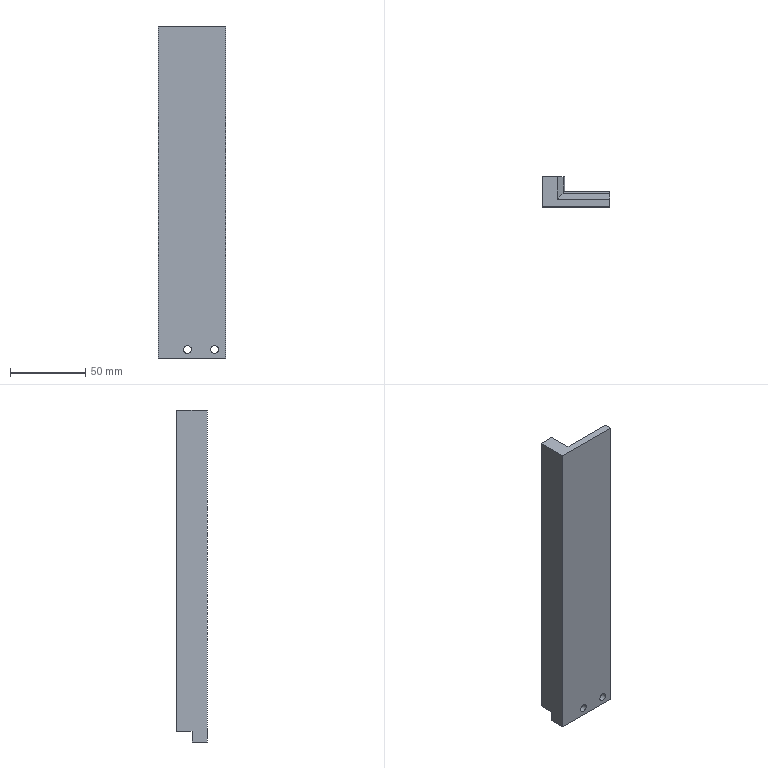Part | STEP file | Tube feed_id110_x_t | 1 solid | 19 faces | box 45 x 20 x 220 mm | volume 129034 mm3 | plane 13 | cylinder 6 | commonest cylinder face diameters 5.2 x2 8.5 x2 20 x2
STEP:
#1=CARTESIAN_POINT('',(0.,0.,0.));
#2=DIRECTION('',(0.,0.,1.));
#3=DIRECTION('',(1.,0.,0.));
#4=AXIS2_PLACEMENT_3D('',#1,#2,#3);
#5=CARTESIAN_POINT('',(-4.,404.936,201.639));
#6=VERTEX_POINT('',#5);
#7=CARTESIAN_POINT('',(-4.,404.936,1.));
#8=VERTEX_POINT('',#7);
#9=CARTESIAN_POINT('',(-4.,404.936,140.));
#10=DIRECTION('',(0.,0.,-1.));
#11=VECTOR('',#10,1.);
#12=LINE('',#9,#11);
#13=CARTESIAN_POINT('',(-4.,411.936,140.));
#14=DIRECTION('',(-1.,0.,0.));
#15=DIRECTION('',(0.,0.,1.));
#16=AXIS2_PLACEMENT_3D('',#13,#14,#15);
#17=PLANE('',#16);
#18=CARTESIAN_POINT('',(0.,-7.));
#19=DIRECTION('',(-1.,0.));
#20=VECTOR('',#19,1.);
#21=LINE('',#18,#20);
#22=(GEOMETRIC_REPRESENTATION_CONTEXT(2)PARAMETRIC_REPRESENTATION_CONTEXT()REPRESENTATION_CONTEXT('',''));
#23=DEFINITIONAL_REPRESENTATION('',(#21),#22);
#24=PCURVE('',#17,#23);
#25=CARTESIAN_POINT('',(-81.505,404.936,329.));
#26=DIRECTION('',(0.,1.,0.));
#27=DIRECTION('',(0.,0.,1.));
#28=AXIS2_PLACEMENT_3D('',#25,#26,#27);
#29=PLANE('',#28);
#30=CARTESIAN_POINT('',(-189.,77.505));
#31=DIRECTION('',(-1.,0.));
#32=VECTOR('',#31,1.);
#33=LINE('',#30,#32);
#34=(GEOMETRIC_REPRESENTATION_CONTEXT(2)PARAMETRIC_REPRESENTATION_CONTEXT()REPRESENTATION_CONTEXT('',''));
#35=DEFINITIONAL_REPRESENTATION('',(#33),#34);
#36=PCURVE('',#29,#35);
#37=SURFACE_CURVE('',#12,(#24,#36),.PCURVE_S1.);
#38=EDGE_CURVE('',#6,#8,#37,.T.);
#39=ORIENTED_EDGE('',*,*,#38,.F.);
#40=CARTESIAN_POINT('',(-4.,394.936,201.639));
#41=VERTEX_POINT('',#40);
#42=CARTESIAN_POINT('',(-4.,394.936,201.639));
#43=DIRECTION('',(0.,-1.,0.));
#44=VECTOR('',#43,1.);
#45=LINE('',#42,#44);
#46=CARTESIAN_POINT('',(61.639,-17.));
#47=DIRECTION('',(0.,-1.));
#48=VECTOR('',#47,1.);
#49=LINE('',#46,#48);
#50=(GEOMETRIC_REPRESENTATION_CONTEXT(2)PARAMETRIC_REPRESENTATION_CONTEXT()REPRESENTATION_CONTEXT('',''));
#51=DEFINITIONAL_REPRESENTATION('',(#49),#50);
#52=PCURVE('',#17,#51);
#53=CARTESIAN_POINT('',(-14.,411.936,201.639));
#54=DIRECTION('',(0.,1.,0.));
#55=DIRECTION('',(-1.,0.,0.));
#56=AXIS2_PLACEMENT_3D('',#53,#54,#55);
#57=CYLINDRICAL_SURFACE('',#56,10.);
#58=CARTESIAN_POINT('',(3.142,-17.));
#59=DIRECTION('',(0.,-1.));
#60=VECTOR('',#59,1.);
#61=LINE('',#58,#60);
#62=(GEOMETRIC_REPRESENTATION_CONTEXT(2)PARAMETRIC_REPRESENTATION_CONTEXT()REPRESENTATION_CONTEXT('',''));
#63=DEFINITIONAL_REPRESENTATION('',(#61),#62);
#64=PCURVE('',#57,#63);
#65=SURFACE_CURVE('',#45,(#52,#64),.PCURVE_S1.);
#66=EDGE_CURVE('',#6,#41,#65,.T.);
#67=ORIENTED_EDGE('',*,*,#66,.T.);
#68=CARTESIAN_POINT('',(-4.,394.936,1.));
#69=VERTEX_POINT('',#68);
#70=CARTESIAN_POINT('',(-4.,394.936,140.));
#71=DIRECTION('',(0.,0.,-1.));
#72=VECTOR('',#71,1.);
#73=LINE('',#70,#72);
#74=CARTESIAN_POINT('',(0.,-17.));
#75=DIRECTION('',(-1.,0.));
#76=VECTOR('',#75,1.);
#77=LINE('',#74,#76);
#78=(GEOMETRIC_REPRESENTATION_CONTEXT(2)PARAMETRIC_REPRESENTATION_CONTEXT()REPRESENTATION_CONTEXT('',''));
#79=DEFINITIONAL_REPRESENTATION('',(#77),#78);
#80=PCURVE('',#17,#79);
#81=CARTESIAN_POINT('',(21.,394.936,140.));
#82=DIRECTION('',(0.,-1.,0.));
#83=DIRECTION('',(0.,0.,-1.));
#84=AXIS2_PLACEMENT_3D('',#81,#82,#83);
#85=PLANE('',#84);
#86=CARTESIAN_POINT('',(0.,-25.));
#87=DIRECTION('',(1.,0.));
#88=VECTOR('',#87,1.);
#89=LINE('',#86,#88);
#90=(GEOMETRIC_REPRESENTATION_CONTEXT(2)PARAMETRIC_REPRESENTATION_CONTEXT()REPRESENTATION_CONTEXT('',''));
#91=DEFINITIONAL_REPRESENTATION('',(#89),#90);
#92=PCURVE('',#85,#91);
#93=SURFACE_CURVE('',#73,(#80,#92),.PCURVE_S1.);
#94=EDGE_CURVE('',#41,#69,#93,.T.);
#95=ORIENTED_EDGE('',*,*,#94,.T.);
#96=CARTESIAN_POINT('',(-4.,0.,1.));
#97=DIRECTION('',(0.,-1.,0.));
#98=VECTOR('',#97,1.);
#99=LINE('',#96,#98);
#100=CARTESIAN_POINT('',(-139.,-411.936));
#101=DIRECTION('',(0.,-1.));
#102=VECTOR('',#101,1.);
#103=LINE('',#100,#102);
#104=(GEOMETRIC_REPRESENTATION_CONTEXT(2)PARAMETRIC_REPRESENTATION_CONTEXT()REPRESENTATION_CONTEXT('',''));
#105=DEFINITIONAL_REPRESENTATION('',(#103),#104);
#106=PCURVE('',#17,#105);
#107=CARTESIAN_POINT('',(0.,0.,1.));
#108=DIRECTION('',(0.,0.,1.));
#109=DIRECTION('',(0.,-1.,0.));
#110=AXIS2_PLACEMENT_3D('',#107,#108,#109);
#111=PLANE('',#110);
#112=CARTESIAN_POINT('',(0.,-4.));
#113=DIRECTION('',(1.,0.));
#114=VECTOR('',#113,1.);
#115=LINE('',#112,#114);
#116=(GEOMETRIC_REPRESENTATION_CONTEXT(2)PARAMETRIC_REPRESENTATION_CONTEXT()REPRESENTATION_CONTEXT('',''));
#117=DEFINITIONAL_REPRESENTATION('',(#115),#116);
#118=PCURVE('',#111,#117);
#119=SURFACE_CURVE('',#99,(#106,#118),.PCURVE_S1.);
#120=EDGE_CURVE('',#8,#69,#119,.T.);
#121=ORIENTED_EDGE('',*,*,#120,.F.);
#122=EDGE_LOOP('',(#39,#67,#95,#121));
#123=FACE_BOUND('',#122,.T.);
#124=ADVANCED_FACE('',(#123),#17,.F.);
#125=CARTESIAN_POINT('',(-19.,394.936,-6.));
#126=VERTEX_POINT('',#125);
#127=CARTESIAN_POINT('',(-19.,384.936,-6.));
#128=VERTEX_POINT('',#127);
#129=CARTESIAN_POINT('',(-19.,439.436,-6.));
#130=DIRECTION('',(0.,-1.,0.));
#131=VECTOR('',#130,1.);
#132=LINE('',#129,#131);
#133=CARTESIAN_POINT('',(0.,0.,-6.));
#134=DIRECTION('',(0.,0.,1.));
#135=DIRECTION('',(0.,-1.,0.));
#136=AXIS2_PLACEMENT_3D('',#133,#134,#135);
#137=PLANE('',#136);
#138=CARTESIAN_POINT('',(-439.436,-19.));
#139=DIRECTION('',(1.,0.));
#140=VECTOR('',#139,1.);
#141=LINE('',#138,#140);
#142=(GEOMETRIC_REPRESENTATION_CONTEXT(2)PARAMETRIC_REPRESENTATION_CONTEXT()REPRESENTATION_CONTEXT('',''));
#143=DEFINITIONAL_REPRESENTATION('',(#141),#142);
#144=PCURVE('',#137,#143);
#145=CARTESIAN_POINT('',(-19.,439.436,140.));
#146=DIRECTION('',(1.,0.,0.));
#147=DIRECTION('',(0.,0.,-1.));
#148=AXIS2_PLACEMENT_3D('',#145,#146,#147);
#149=PLANE('',#148);
#150=CARTESIAN_POINT('',(146.,0.));
#151=DIRECTION('',(0.,-1.));
#152=VECTOR('',#151,1.);
#153=LINE('',#150,#152);
#154=(GEOMETRIC_REPRESENTATION_CONTEXT(2)PARAMETRIC_REPRESENTATION_CONTEXT()REPRESENTATION_CONTEXT('',''));
#155=DEFINITIONAL_REPRESENTATION('',(#153),#154);
#156=PCURVE('',#149,#155);
#157=SURFACE_CURVE('',#132,(#144,#156),.PCURVE_S1.);
#158=EDGE_CURVE('',#126,#128,#157,.T.);
#159=ORIENTED_EDGE('',*,*,#158,.F.);
#160=CARTESIAN_POINT('',(26.,394.936,-6.));
#161=VERTEX_POINT('',#160);
#162=CARTESIAN_POINT('',(21.,394.936,-6.));
#163=DIRECTION('',(-1.,0.,0.));
#164=VECTOR('',#163,1.);
#165=LINE('',#162,#164);
#166=CARTESIAN_POINT('',(-394.936,21.));
#167=DIRECTION('',(0.,-1.));
#168=VECTOR('',#167,1.);
#169=LINE('',#166,#168);
#170=(GEOMETRIC_REPRESENTATION_CONTEXT(2)PARAMETRIC_REPRESENTATION_CONTEXT()REPRESENTATION_CONTEXT('',''));
#171=DEFINITIONAL_REPRESENTATION('',(#169),#170);
#172=PCURVE('',#137,#171);
#173=CARTESIAN_POINT('',(146.,0.));
#174=DIRECTION('',(0.,-1.));
#175=VECTOR('',#174,1.);
#176=LINE('',#173,#175);
#177=(GEOMETRIC_REPRESENTATION_CONTEXT(2)PARAMETRIC_REPRESENTATION_CONTEXT()REPRESENTATION_CONTEXT('',''));
#178=DEFINITIONAL_REPRESENTATION('',(#176),#177);
#179=PCURVE('',#85,#178);
#180=SURFACE_CURVE('',#165,(#172,#179),.PCURVE_S1.);
#181=EDGE_CURVE('',#161,#126,#180,.T.);
#182=ORIENTED_EDGE('',*,*,#181,.F.);
#183=CARTESIAN_POINT('',(26.,384.936,-6.));
#184=VERTEX_POINT('',#183);
#185=CARTESIAN_POINT('',(26.,384.436,-6.));
#186=DIRECTION('',(0.,1.,0.));
#187=VECTOR('',#186,1.);
#188=LINE('',#185,#187);
#189=CARTESIAN_POINT('',(-384.436,26.));
#190=DIRECTION('',(-1.,0.));
#191=VECTOR('',#190,1.);
#192=LINE('',#189,#191);
#193=(GEOMETRIC_REPRESENTATION_CONTEXT(2)PARAMETRIC_REPRESENTATION_CONTEXT()REPRESENTATION_CONTEXT('',''));
#194=DEFINITIONAL_REPRESENTATION('',(#192),#193);
#195=PCURVE('',#137,#194);
#196=CARTESIAN_POINT('',(26.,384.436,140.));
#197=DIRECTION('',(-1.,0.,0.));
#198=DIRECTION('',(0.,0.,1.));
#199=AXIS2_PLACEMENT_3D('',#196,#197,#198);
#200=PLANE('',#199);
#201=CARTESIAN_POINT('',(-146.,0.));
#202=DIRECTION('',(0.,1.));
#203=VECTOR('',#202,1.);
#204=LINE('',#201,#203);
#205=(GEOMETRIC_REPRESENTATION_CONTEXT(2)PARAMETRIC_REPRESENTATION_CONTEXT()REPRESENTATION_CONTEXT('',''));
#206=DEFINITIONAL_REPRESENTATION('',(#204),#205);
#207=PCURVE('',#200,#206);
#208=SURFACE_CURVE('',#188,(#195,#207),.PCURVE_S1.);
#209=EDGE_CURVE('',#184,#161,#208,.T.);
#210=ORIENTED_EDGE('',*,*,#209,.F.);
#211=CARTESIAN_POINT('',(-19.,384.936,-6.));
#212=DIRECTION('',(1.,0.,0.));
#213=VECTOR('',#212,1.);
#214=LINE('',#211,#213);
#215=CARTESIAN_POINT('',(-384.936,-19.));
#216=DIRECTION('',(0.,1.));
#217=VECTOR('',#216,1.);
#218=LINE('',#215,#217);
#219=(GEOMETRIC_REPRESENTATION_CONTEXT(2)PARAMETRIC_REPRESENTATION_CONTEXT()REPRESENTATION_CONTEXT('',''));
#220=DEFINITIONAL_REPRESENTATION('',(#218),#219);
#221=PCURVE('',#137,#220);
#222=CARTESIAN_POINT('',(-19.,384.936,140.));
#223=DIRECTION('',(0.,1.,0.));
#224=DIRECTION('',(-1.,0.,0.));
#225=AXIS2_PLACEMENT_3D('',#222,#223,#224);
#226=PLANE('',#225);
#227=CARTESIAN_POINT('',(0.,-146.));
#228=DIRECTION('',(-1.,0.));
#229=VECTOR('',#228,1.);
#230=LINE('',#227,#229);
#231=(GEOMETRIC_REPRESENTATION_CONTEXT(2)PARAMETRIC_REPRESENTATION_CONTEXT()REPRESENTATION_CONTEXT('',''));
#232=DEFINITIONAL_REPRESENTATION('',(#230),#231);
#233=PCURVE('',#226,#232);
#234=SURFACE_CURVE('',#214,(#221,#233),.PCURVE_S1.);
#235=EDGE_CURVE('',#128,#184,#234,.T.);
#236=ORIENTED_EDGE('',*,*,#235,.F.);
#237=EDGE_LOOP('',(#159,#182,#210,#236));
#238=FACE_BOUND('',#237,.T.);
#239=ADVANCED_FACE('',(#238),#137,.F.);
#240=CARTESIAN_POINT('',(26.,384.936,214.));
#241=VERTEX_POINT('',#240);
#242=CARTESIAN_POINT('',(26.,389.936,214.));
#243=VERTEX_POINT('',#242);
#244=CARTESIAN_POINT('',(26.,384.436,214.));
#245=DIRECTION('',(0.,1.,0.));
#246=VECTOR('',#245,1.);
#247=LINE('',#244,#246);
#248=CARTESIAN_POINT('',(0.,0.,214.));
#249=DIRECTION('',(0.,0.,1.));
#250=DIRECTION('',(0.,-1.,0.));
#251=AXIS2_PLACEMENT_3D('',#248,#249,#250);
#252=PLANE('',#251);
#253=CARTESIAN_POINT('',(-384.436,26.));
#254=DIRECTION('',(-1.,0.));
#255=VECTOR('',#254,1.);
#256=LINE('',#253,#255);
#257=(GEOMETRIC_REPRESENTATION_CONTEXT(2)PARAMETRIC_REPRESENTATION_CONTEXT()REPRESENTATION_CONTEXT('',''));
#258=DEFINITIONAL_REPRESENTATION('',(#256),#257);
#259=PCURVE('',#252,#258);
#260=CARTESIAN_POINT('',(74.,0.));
#261=DIRECTION('',(0.,1.));
#262=VECTOR('',#261,1.);
#263=LINE('',#260,#262);
#264=(GEOMETRIC_REPRESENTATION_CONTEXT(2)PARAMETRIC_REPRESENTATION_CONTEXT()REPRESENTATION_CONTEXT('',''));
#265=DEFINITIONAL_REPRESENTATION('',(#263),#264);
#266=PCURVE('',#200,#265);
#267=SURFACE_CURVE('',#247,(#259,#266),.PCURVE_S1.);
#268=EDGE_CURVE('',#241,#243,#267,.T.);
#269=ORIENTED_EDGE('',*,*,#268,.T.);
#270=CARTESIAN_POINT('',(-9.,389.936,214.));
#271=VERTEX_POINT('',#270);
#272=CARTESIAN_POINT('',(-4.,389.936,214.));
#273=DIRECTION('',(-1.,0.,0.));
#274=VECTOR('',#273,1.);
#275=LINE('',#272,#274);
#276=CARTESIAN_POINT('',(-389.936,-4.));
#277=DIRECTION('',(0.,-1.));
#278=VECTOR('',#277,1.);
#279=LINE('',#276,#278);
#280=(GEOMETRIC_REPRESENTATION_CONTEXT(2)PARAMETRIC_REPRESENTATION_CONTEXT()REPRESENTATION_CONTEXT('',''));
#281=DEFINITIONAL_REPRESENTATION('',(#279),#280);
#282=PCURVE('',#252,#281);
#283=CARTESIAN_POINT('',(0.,389.936,214.));
#284=DIRECTION('',(0.,0.8944,0.4472));
#285=DIRECTION('',(1.,0.,0.));
#286=AXIS2_PLACEMENT_3D('',#283,#284,#285);
#287=PLANE('',#286);
#288=CARTESIAN_POINT('',(-4.,0.));
#289=DIRECTION('',(-1.,0.));
#290=VECTOR('',#289,1.);
#291=LINE('',#288,#290);
#292=(GEOMETRIC_REPRESENTATION_CONTEXT(2)PARAMETRIC_REPRESENTATION_CONTEXT()REPRESENTATION_CONTEXT('',''));
#293=DEFINITIONAL_REPRESENTATION('',(#291),#292);
#294=PCURVE('',#287,#293);
#295=SURFACE_CURVE('',#275,(#282,#294),.PCURVE_S1.);
#296=EDGE_CURVE('',#243,#271,#295,.T.);
#297=ORIENTED_EDGE('',*,*,#296,.T.);
#298=CARTESIAN_POINT('',(-9.,404.936,214.));
#299=VERTEX_POINT('',#298);
#300=CARTESIAN_POINT('',(-9.,400.936,214.));
#301=DIRECTION('',(0.,1.,0.));
#302=VECTOR('',#301,1.);
#303=LINE('',#300,#302);
#304=CARTESIAN_POINT('',(-400.936,-9.));
#305=DIRECTION('',(-1.,0.));
#306=VECTOR('',#305,1.);
#307=LINE('',#304,#306);
#308=(GEOMETRIC_REPRESENTATION_CONTEXT(2)PARAMETRIC_REPRESENTATION_CONTEXT()REPRESENTATION_CONTEXT('',''));
#309=DEFINITIONAL_REPRESENTATION('',(#307),#308);
#310=PCURVE('',#252,#309);
#311=CARTESIAN_POINT('',(-9.,0.,214.));
#312=DIRECTION('',(0.8944,0.,0.4472));
#313=DIRECTION('',(0.,-1.,0.));
#314=AXIS2_PLACEMENT_3D('',#311,#312,#313);
#315=PLANE('',#314);
#316=CARTESIAN_POINT('',(-400.936,0.));
#317=DIRECTION('',(-1.,0.));
#318=VECTOR('',#317,1.);
#319=LINE('',#316,#318);
#320=(GEOMETRIC_REPRESENTATION_CONTEXT(2)PARAMETRIC_REPRESENTATION_CONTEXT()REPRESENTATION_CONTEXT('',''));
#321=DEFINITIONAL_REPRESENTATION('',(#319),#320);
#322=PCURVE('',#315,#321);
#323=SURFACE_CURVE('',#303,(#310,#322),.PCURVE_S1.);
#324=EDGE_CURVE('',#271,#299,#323,.T.);
#325=ORIENTED_EDGE('',*,*,#324,.T.);
#326=CARTESIAN_POINT('',(-19.,404.936,214.));
#327=VERTEX_POINT('',#326);
#328=CARTESIAN_POINT('',(0.,404.936,214.));
#329=DIRECTION('',(-1.,0.,0.));
#330=VECTOR('',#329,1.);
#331=LINE('',#328,#330);
#332=CARTESIAN_POINT('',(-404.936,0.));
#333=DIRECTION('',(0.,-1.));
#334=VECTOR('',#333,1.);
#335=LINE('',#332,#334);
#336=(GEOMETRIC_REPRESENTATION_CONTEXT(2)PARAMETRIC_REPRESENTATION_CONTEXT()REPRESENTATION_CONTEXT('',''));
#337=DEFINITIONAL_REPRESENTATION('',(#335),#336);
#338=PCURVE('',#252,#337);
#339=CARTESIAN_POINT('',(-115.,81.505));
#340=DIRECTION('',(0.,-1.));
#341=VECTOR('',#340,1.);
#342=LINE('',#339,#341);
#343=(GEOMETRIC_REPRESENTATION_CONTEXT(2)PARAMETRIC_REPRESENTATION_CONTEXT()REPRESENTATION_CONTEXT('',''));
#344=DEFINITIONAL_REPRESENTATION('',(#342),#343);
#345=PCURVE('',#29,#344);
#346=SURFACE_CURVE('',#331,(#338,#345),.PCURVE_S1.);
#347=EDGE_CURVE('',#299,#327,#346,.T.);
#348=ORIENTED_EDGE('',*,*,#347,.T.);
#349=CARTESIAN_POINT('',(-19.,384.936,214.));
#350=VERTEX_POINT('',#349);
#351=CARTESIAN_POINT('',(-19.,439.436,214.));
#352=DIRECTION('',(0.,-1.,0.));
#353=VECTOR('',#352,1.);
#354=LINE('',#351,#353);
#355=CARTESIAN_POINT('',(-439.436,-19.));
#356=DIRECTION('',(1.,0.));
#357=VECTOR('',#356,1.);
#358=LINE('',#355,#357);
#359=(GEOMETRIC_REPRESENTATION_CONTEXT(2)PARAMETRIC_REPRESENTATION_CONTEXT()REPRESENTATION_CONTEXT('',''));
#360=DEFINITIONAL_REPRESENTATION('',(#358),#359);
#361=PCURVE('',#252,#360);
#362=CARTESIAN_POINT('',(-74.,0.));
#363=DIRECTION('',(0.,-1.));
#364=VECTOR('',#363,1.);
#365=LINE('',#362,#364);
#366=(GEOMETRIC_REPRESENTATION_CONTEXT(2)PARAMETRIC_REPRESENTATION_CONTEXT()REPRESENTATION_CONTEXT('',''));
#367=DEFINITIONAL_REPRESENTATION('',(#365),#366);
#368=PCURVE('',#149,#367);
#369=SURFACE_CURVE('',#354,(#361,#368),.PCURVE_S1.);
#370=EDGE_CURVE('',#327,#350,#369,.T.);
#371=ORIENTED_EDGE('',*,*,#370,.T.);
#372=CARTESIAN_POINT('',(-19.,384.936,214.));
#373=DIRECTION('',(1.,0.,0.));
#374=VECTOR('',#373,1.);
#375=LINE('',#372,#374);
#376=CARTESIAN_POINT('',(-384.936,-19.));
#377=DIRECTION('',(0.,1.));
#378=VECTOR('',#377,1.);
#379=LINE('',#376,#378);
#380=(GEOMETRIC_REPRESENTATION_CONTEXT(2)PARAMETRIC_REPRESENTATION_CONTEXT()REPRESENTATION_CONTEXT('',''));
#381=DEFINITIONAL_REPRESENTATION('',(#379),#380);
#382=PCURVE('',#252,#381);
#383=CARTESIAN_POINT('',(0.,74.));
#384=DIRECTION('',(-1.,0.));
#385=VECTOR('',#384,1.);
#386=LINE('',#383,#385);
#387=(GEOMETRIC_REPRESENTATION_CONTEXT(2)PARAMETRIC_REPRESENTATION_CONTEXT()REPRESENTATION_CONTEXT('',''));
#388=DEFINITIONAL_REPRESENTATION('',(#386),#387);
#389=PCURVE('',#226,#388);
#390=SURFACE_CURVE('',#375,(#382,#389),.PCURVE_S1.);
#391=EDGE_CURVE('',#350,#241,#390,.T.);
#392=ORIENTED_EDGE('',*,*,#391,.T.);
#393=EDGE_LOOP('',(#269,#297,#325,#348,#371,#392));
#394=FACE_BOUND('',#393,.T.);
#395=ADVANCED_FACE('',(#394),#252,.T.);
#396=CARTESIAN_POINT('',(-19.,404.936,1.));
#397=VERTEX_POINT('',#396);
#398=CARTESIAN_POINT('',(-19.,404.936,140.));
#399=DIRECTION('',(0.,0.,1.));
#400=VECTOR('',#399,1.);
#401=LINE('',#398,#400);
#402=CARTESIAN_POINT('',(0.,-34.5));
#403=DIRECTION('',(-1.,0.));
#404=VECTOR('',#403,1.);
#405=LINE('',#402,#404);
#406=(GEOMETRIC_REPRESENTATION_CONTEXT(2)PARAMETRIC_REPRESENTATION_CONTEXT()REPRESENTATION_CONTEXT('',''));
#407=DEFINITIONAL_REPRESENTATION('',(#405),#406);
#408=PCURVE('',#149,#407);
#409=CARTESIAN_POINT('',(-189.,62.505));
#410=DIRECTION('',(1.,0.));
#411=VECTOR('',#410,1.);
#412=LINE('',#409,#411);
#413=(GEOMETRIC_REPRESENTATION_CONTEXT(2)PARAMETRIC_REPRESENTATION_CONTEXT()REPRESENTATION_CONTEXT('',''));
#414=DEFINITIONAL_REPRESENTATION('',(#412),#413);
#415=PCURVE('',#29,#414);
#416=SURFACE_CURVE('',#401,(#408,#415),.PCURVE_S1.);
#417=EDGE_CURVE('',#397,#327,#416,.T.);
#418=ORIENTED_EDGE('',*,*,#417,.F.);
#419=CARTESIAN_POINT('',(-19.,394.936,1.));
#420=VERTEX_POINT('',#419);
#421=CARTESIAN_POINT('',(-19.,439.436,1.));
#422=DIRECTION('',(0.,-1.,0.));
#423=VECTOR('',#422,1.);
#424=LINE('',#421,#423);
#425=CARTESIAN_POINT('',(139.,0.));
#426=DIRECTION('',(0.,-1.));
#427=VECTOR('',#426,1.);
#428=LINE('',#425,#427);
#429=(GEOMETRIC_REPRESENTATION_CONTEXT(2)PARAMETRIC_REPRESENTATION_CONTEXT()REPRESENTATION_CONTEXT('',''));
#430=DEFINITIONAL_REPRESENTATION('',(#428),#429);
#431=PCURVE('',#149,#430);
#432=CARTESIAN_POINT('',(-439.436,-19.));
#433=DIRECTION('',(1.,0.));
#434=VECTOR('',#433,1.);
#435=LINE('',#432,#434);
#436=(GEOMETRIC_REPRESENTATION_CONTEXT(2)PARAMETRIC_REPRESENTATION_CONTEXT()REPRESENTATION_CONTEXT('',''));
#437=DEFINITIONAL_REPRESENTATION('',(#435),#436);
#438=PCURVE('',#111,#437);
#439=SURFACE_CURVE('',#424,(#431,#438),.PCURVE_S1.);
#440=EDGE_CURVE('',#397,#420,#439,.T.);
#441=ORIENTED_EDGE('',*,*,#440,.T.);
#442=CARTESIAN_POINT('',(-19.,394.936,140.));
#443=DIRECTION('',(0.,0.,-1.));
#444=VECTOR('',#443,1.);
#445=LINE('',#442,#444);
#446=CARTESIAN_POINT('',(0.,-44.5));
#447=DIRECTION('',(1.,0.));
#448=VECTOR('',#447,1.);
#449=LINE('',#446,#448);
#450=(GEOMETRIC_REPRESENTATION_CONTEXT(2)PARAMETRIC_REPRESENTATION_CONTEXT()REPRESENTATION_CONTEXT('',''));
#451=DEFINITIONAL_REPRESENTATION('',(#449),#450);
#452=PCURVE('',#149,#451);
#453=CARTESIAN_POINT('',(0.,-40.));
#454=DIRECTION('',(1.,0.));
#455=VECTOR('',#454,1.);
#456=LINE('',#453,#455);
#457=(GEOMETRIC_REPRESENTATION_CONTEXT(2)PARAMETRIC_REPRESENTATION_CONTEXT()REPRESENTATION_CONTEXT('',''));
#458=DEFINITIONAL_REPRESENTATION('',(#456),#457);
#459=PCURVE('',#85,#458);
#460=SURFACE_CURVE('',#445,(#452,#459),.PCURVE_S1.);
#461=EDGE_CURVE('',#420,#126,#460,.T.);
#462=ORIENTED_EDGE('',*,*,#461,.T.);
#463=ORIENTED_EDGE('',*,*,#158,.T.);
#464=CARTESIAN_POINT('',(-19.,384.936,140.));
#465=DIRECTION('',(0.,0.,1.));
#466=VECTOR('',#465,1.);
#467=LINE('',#464,#466);
#468=CARTESIAN_POINT('',(0.,-54.5));
#469=DIRECTION('',(-1.,0.));
#470=VECTOR('',#469,1.);
#471=LINE('',#468,#470);
#472=(GEOMETRIC_REPRESENTATION_CONTEXT(2)PARAMETRIC_REPRESENTATION_CONTEXT()REPRESENTATION_CONTEXT('',''));
#473=DEFINITIONAL_REPRESENTATION('',(#471),#472);
#474=PCURVE('',#149,#473);
#475=CARTESIAN_POINT('',(0.,0.));
#476=DIRECTION('',(0.,1.));
#477=VECTOR('',#476,1.);
#478=LINE('',#475,#477);
#479=(GEOMETRIC_REPRESENTATION_CONTEXT(2)PARAMETRIC_REPRESENTATION_CONTEXT()REPRESENTATION_CONTEXT('',''));
#480=DEFINITIONAL_REPRESENTATION('',(#478),#479);
#481=PCURVE('',#226,#480);
#482=SURFACE_CURVE('',#467,(#474,#481),.PCURVE_S1.);
#483=EDGE_CURVE('',#128,#350,#482,.T.);
#484=ORIENTED_EDGE('',*,*,#483,.T.);
#485=ORIENTED_EDGE('',*,*,#370,.F.);
#486=EDGE_LOOP('',(#418,#441,#462,#463,#484,#485));
#487=FACE_BOUND('',#486,.T.);
#488=ADVANCED_FACE('',(#487),#149,.F.);
#489=CARTESIAN_POINT('',(3.1,384.936,-0.5));
#490=VERTEX_POINT('',#489);
#491=CARTESIAN_POINT('',(0.5,384.936,2.1));
#492=VERTEX_POINT('',#491);
#493=CARTESIAN_POINT('',(0.5,384.936,-0.5));
#494=DIRECTION('',(0.,1.,0.));
#495=DIRECTION('',(1.,0.,0.));
#496=AXIS2_PLACEMENT_3D('',#493,#494,#495);
#497=CIRCLE('',#496,2.6);
#498=CARTESIAN_POINT('',(-19.5,-140.5));
#499=DIRECTION('',(-1.,0.));
#500=AXIS2_PLACEMENT_2D('',#498,#499);
#501=CIRCLE('',#500,2.6);
#502=(GEOMETRIC_REPRESENTATION_CONTEXT(2)PARAMETRIC_REPRESENTATION_CONTEXT()REPRESENTATION_CONTEXT('',''));
#503=DEFINITIONAL_REPRESENTATION('',(#501),#502);
#504=PCURVE('',#226,#503);
#505=CARTESIAN_POINT('',(0.5,374.936,-0.5));
#506=DIRECTION('',(0.,-1.,0.));
#507=DIRECTION('',(0.,0.,1.));
#508=AXIS2_PLACEMENT_3D('',#505,#506,#507);
#509=CYLINDRICAL_SURFACE('',#508,2.6);
#510=CARTESIAN_POINT('',(4.712,-10.));
#511=DIRECTION('',(-1.,0.));
#512=VECTOR('',#511,1.);
#513=LINE('',#510,#512);
#514=(GEOMETRIC_REPRESENTATION_CONTEXT(2)PARAMETRIC_REPRESENTATION_CONTEXT()REPRESENTATION_CONTEXT('',''));
#515=DEFINITIONAL_REPRESENTATION('',(#513),#514);
#516=PCURVE('',#509,#515);
#517=SURFACE_CURVE('',#497,(#504,#516),.PCURVE_S1.);
#518=EDGE_CURVE('',#490,#492,#517,.T.);
#519=ORIENTED_EDGE('',*,*,#518,.T.);
#520=CARTESIAN_POINT('',(0.5,384.936,-0.5));
#521=DIRECTION('',(0.,1.,0.));
#522=DIRECTION('',(1.,0.,0.));
#523=AXIS2_PLACEMENT_3D('',#520,#521,#522);
#524=CIRCLE('',#523,2.6);
#525=CARTESIAN_POINT('',(-19.5,-140.5));
#526=DIRECTION('',(-1.,0.));
#527=AXIS2_PLACEMENT_2D('',#525,#526);
#528=CIRCLE('',#527,2.6);
#529=(GEOMETRIC_REPRESENTATION_CONTEXT(2)PARAMETRIC_REPRESENTATION_CONTEXT()REPRESENTATION_CONTEXT('',''));
#530=DEFINITIONAL_REPRESENTATION('',(#528),#529);
#531=PCURVE('',#226,#530);
#532=CARTESIAN_POINT('',(10.996,-10.));
#533=DIRECTION('',(-1.,0.));
#534=VECTOR('',#533,1.);
#535=LINE('',#532,#534);
#536=(GEOMETRIC_REPRESENTATION_CONTEXT(2)PARAMETRIC_REPRESENTATION_CONTEXT()REPRESENTATION_CONTEXT('',''));
#537=DEFINITIONAL_REPRESENTATION('',(#535),#536);
#538=PCURVE('',#509,#537);
#539=SURFACE_CURVE('',#524,(#531,#538),.PCURVE_S1.);
#540=EDGE_CURVE('',#492,#490,#539,.T.);
#541=ORIENTED_EDGE('',*,*,#540,.T.);
#542=EDGE_LOOP('',(#519,#541));
#543=FACE_BOUND('',#542,.T.);
#544=CARTESIAN_POINT('',(21.1,384.936,-0.5));
#545=VERTEX_POINT('',#544);
#546=CARTESIAN_POINT('',(18.5,384.936,2.1));
#547=VERTEX_POINT('',#546);
#548=CARTESIAN_POINT('',(18.5,384.936,-0.5));
#549=DIRECTION('',(0.,1.,0.));
#550=DIRECTION('',(1.,0.,0.));
#551=AXIS2_PLACEMENT_3D('',#548,#549,#550);
#552=CIRCLE('',#551,2.6);
#553=CARTESIAN_POINT('',(-37.5,-140.5));
#554=DIRECTION('',(-1.,0.));
#555=AXIS2_PLACEMENT_2D('',#553,#554);
#556=CIRCLE('',#555,2.6);
#557=(GEOMETRIC_REPRESENTATION_CONTEXT(2)PARAMETRIC_REPRESENTATION_CONTEXT()REPRESENTATION_CONTEXT('',''));
#558=DEFINITIONAL_REPRESENTATION('',(#556),#557);
#559=PCURVE('',#226,#558);
#560=CARTESIAN_POINT('',(18.5,374.936,-0.5));
#561=DIRECTION('',(0.,-1.,0.));
#562=DIRECTION('',(0.,0.,1.));
#563=AXIS2_PLACEMENT_3D('',#560,#561,#562);
#564=CYLINDRICAL_SURFACE('',#563,2.6);
#565=CARTESIAN_POINT('',(4.712,-10.));
#566=DIRECTION('',(-1.,0.));
#567=VECTOR('',#566,1.);
#568=LINE('',#565,#567);
#569=(GEOMETRIC_REPRESENTATION_CONTEXT(2)PARAMETRIC_REPRESENTATION_CONTEXT()REPRESENTATION_CONTEXT('',''));
#570=DEFINITIONAL_REPRESENTATION('',(#568),#569);
#571=PCURVE('',#564,#570);
#572=SURFACE_CURVE('',#552,(#559,#571),.PCURVE_S1.);
#573=EDGE_CURVE('',#545,#547,#572,.T.);
#574=ORIENTED_EDGE('',*,*,#573,.T.);
#575=CARTESIAN_POINT('',(18.5,384.936,-0.5));
#576=DIRECTION('',(0.,1.,0.));
#577=DIRECTION('',(1.,0.,0.));
#578=AXIS2_PLACEMENT_3D('',#575,#576,#577);
#579=CIRCLE('',#578,2.6);
#580=CARTESIAN_POINT('',(-37.5,-140.5));
#581=DIRECTION('',(-1.,0.));
#582=AXIS2_PLACEMENT_2D('',#580,#581);
#583=CIRCLE('',#582,2.6);
#584=(GEOMETRIC_REPRESENTATION_CONTEXT(2)PARAMETRIC_REPRESENTATION_CONTEXT()REPRESENTATION_CONTEXT('',''));
#585=DEFINITIONAL_REPRESENTATION('',(#583),#584);
#586=PCURVE('',#226,#585);
#587=CARTESIAN_POINT('',(10.996,-10.));
#588=DIRECTION('',(-1.,0.));
#589=VECTOR('',#588,1.);
#590=LINE('',#587,#589);
#591=(GEOMETRIC_REPRESENTATION_CONTEXT(2)PARAMETRIC_REPRESENTATION_CONTEXT()REPRESENTATION_CONTEXT('',''));
#592=DEFINITIONAL_REPRESENTATION('',(#590),#591);
#593=PCURVE('',#564,#592);
#594=SURFACE_CURVE('',#579,(#586,#593),.PCURVE_S1.);
#595=EDGE_CURVE('',#547,#545,#594,.T.);
#596=ORIENTED_EDGE('',*,*,#595,.T.);
#597=EDGE_LOOP('',(#574,#596));
#598=FACE_BOUND('',#597,.T.);
#599=ORIENTED_EDGE('',*,*,#391,.F.);
#600=ORIENTED_EDGE('',*,*,#483,.F.);
#601=ORIENTED_EDGE('',*,*,#235,.T.);
#602=CARTESIAN_POINT('',(26.,384.936,140.));
#603=DIRECTION('',(0.,0.,1.));
#604=VECTOR('',#603,1.);
#605=LINE('',#602,#604);
#606=CARTESIAN_POINT('',(-45.,0.));
#607=DIRECTION('',(0.,1.));
#608=VECTOR('',#607,1.);
#609=LINE('',#606,#608);
#610=(GEOMETRIC_REPRESENTATION_CONTEXT(2)PARAMETRIC_REPRESENTATION_CONTEXT()REPRESENTATION_CONTEXT('',''));
#611=DEFINITIONAL_REPRESENTATION('',(#609),#610);
#612=PCURVE('',#226,#611);
#613=CARTESIAN_POINT('',(0.,0.5));
#614=DIRECTION('',(1.,0.));
#615=VECTOR('',#614,1.);
#616=LINE('',#613,#615);
#617=(GEOMETRIC_REPRESENTATION_CONTEXT(2)PARAMETRIC_REPRESENTATION_CONTEXT()REPRESENTATION_CONTEXT('',''));
#618=DEFINITIONAL_REPRESENTATION('',(#616),#617);
#619=PCURVE('',#200,#618);
#620=SURFACE_CURVE('',#605,(#612,#619),.PCURVE_S1.);
#621=EDGE_CURVE('',#184,#241,#620,.T.);
#622=ORIENTED_EDGE('',*,*,#621,.T.);
#623=EDGE_LOOP('',(#599,#600,#601,#622));
#624=FACE_BOUND('',#623,.T.);
#625=ADVANCED_FACE('',(#543,#598,#624),#226,.F.);
#626=CARTESIAN_POINT('',(26.,394.936,201.639));
#627=VERTEX_POINT('',#626);
#628=CARTESIAN_POINT('',(26.,394.936,140.));
#629=DIRECTION('',(0.,0.,-1.));
#630=VECTOR('',#629,1.);
#631=LINE('',#628,#630);
#632=CARTESIAN_POINT('',(0.,10.5));
#633=DIRECTION('',(-1.,0.));
#634=VECTOR('',#633,1.);
#635=LINE('',#632,#634);
#636=(GEOMETRIC_REPRESENTATION_CONTEXT(2)PARAMETRIC_REPRESENTATION_CONTEXT()REPRESENTATION_CONTEXT('',''));
#637=DEFINITIONAL_REPRESENTATION('',(#635),#636);
#638=PCURVE('',#200,#637);
#639=CARTESIAN_POINT('',(0.,5.));
#640=DIRECTION('',(1.,0.));
#641=VECTOR('',#640,1.);
#642=LINE('',#639,#641);
#643=(GEOMETRIC_REPRESENTATION_CONTEXT(2)PARAMETRIC_REPRESENTATION_CONTEXT()REPRESENTATION_CONTEXT('',''));
#644=DEFINITIONAL_REPRESENTATION('',(#642),#643);
#645=PCURVE('',#85,#644);
#646=SURFACE_CURVE('',#631,(#638,#645),.PCURVE_S1.);
#647=EDGE_CURVE('',#627,#161,#646,.T.);
#648=ORIENTED_EDGE('',*,*,#647,.F.);
#649=CARTESIAN_POINT('',(26.,393.88,206.111));
#650=VERTEX_POINT('',#649);
#651=CARTESIAN_POINT('',(26.,384.936,201.639));
#652=DIRECTION('',(1.,0.,0.));
#653=DIRECTION('',(0.,-1.,0.));
#654=AXIS2_PLACEMENT_3D('',#651,#652,#653);
#655=CIRCLE('',#654,10.);
#656=CARTESIAN_POINT('',(61.639,-9.5));
#657=CARTESIAN_POINT('',(44.319,-9.5));
#658=CARTESIAN_POINT('',(52.979,5.5));
#659=CARTESIAN_POINT('',(61.639,20.5));
#660=CARTESIAN_POINT('',(70.3,5.5));
#661=CARTESIAN_POINT('',(78.96,-9.5));
#662=CARTESIAN_POINT('',(61.639,-9.5));
#663=(BOUNDED_CURVE()B_SPLINE_CURVE(2,(#656,#657,#658,#659,#660,#661,#662),.UNSPECIFIED.,.T.,.F.)B_SPLINE_CURVE_WITH_KNOTS((1,2,2,2,2,1),(-2.094,0.,2.094,4.189,6.283,8.378),.UNSPECIFIED.)CURVE()GEOMETRIC_REPRESENTATION_ITEM()RATIONAL_B_SPLINE_CURVE((1.,0.5,1.,0.5,1.,0.5,1.))REPRESENTATION_ITEM(''));
#664=(GEOMETRIC_REPRESENTATION_CONTEXT(2)PARAMETRIC_REPRESENTATION_CONTEXT()REPRESENTATION_CONTEXT('',''));
#665=DEFINITIONAL_REPRESENTATION('',(#663),#664);
#666=PCURVE('',#200,#665);
#667=CARTESIAN_POINT('',(21.,384.936,201.639));
#668=DIRECTION('',(-1.,0.,0.));
#669=DIRECTION('',(0.,-1.,0.));
#670=AXIS2_PLACEMENT_3D('',#667,#668,#669);
#671=CYLINDRICAL_SURFACE('',#670,10.);
#672=CARTESIAN_POINT('',(6.283,-5.));
#673=DIRECTION('',(-1.,0.));
#674=VECTOR('',#673,1.);
#675=LINE('',#672,#674);
#676=(GEOMETRIC_REPRESENTATION_CONTEXT(2)PARAMETRIC_REPRESENTATION_CONTEXT()REPRESENTATION_CONTEXT('',''));
#677=DEFINITIONAL_REPRESENTATION('',(#675),#676);
#678=PCURVE('',#671,#677);
#679=SURFACE_CURVE('',#655,(#666,#678),.PCURVE_S1.);
#680=EDGE_CURVE('',#627,#650,#679,.T.);
#681=ORIENTED_EDGE('',*,*,#680,.T.);
#682=CARTESIAN_POINT('',(26.,389.936,214.));
#683=DIRECTION('',(0.,-0.4472,0.8944));
#684=VECTOR('',#683,1.);
#685=LINE('',#682,#684);
#686=CARTESIAN_POINT('',(74.,5.5));
#687=DIRECTION('',(0.8944,-0.4472));
#688=VECTOR('',#687,1.);
#689=LINE('',#686,#688);
#690=(GEOMETRIC_REPRESENTATION_CONTEXT(2)PARAMETRIC_REPRESENTATION_CONTEXT()REPRESENTATION_CONTEXT('',''));
#691=DEFINITIONAL_REPRESENTATION('',(#689),#690);
#692=PCURVE('',#200,#691);
#693=CARTESIAN_POINT('',(26.,0.));
#694=DIRECTION('',(0.,-1.));
#695=VECTOR('',#694,1.);
#696=LINE('',#693,#695);
#697=(GEOMETRIC_REPRESENTATION_CONTEXT(2)PARAMETRIC_REPRESENTATION_CONTEXT()REPRESENTATION_CONTEXT('',''));
#698=DEFINITIONAL_REPRESENTATION('',(#696),#697);
#699=PCURVE('',#287,#698);
#700=SURFACE_CURVE('',#685,(#692,#699),.PCURVE_S1.);
#701=EDGE_CURVE('',#650,#243,#700,.T.);
#702=ORIENTED_EDGE('',*,*,#701,.T.);
#703=ORIENTED_EDGE('',*,*,#268,.F.);
#704=ORIENTED_EDGE('',*,*,#621,.F.);
#705=ORIENTED_EDGE('',*,*,#209,.T.);
#706=EDGE_LOOP('',(#648,#681,#702,#703,#704,#705));
#707=FACE_BOUND('',#706,.T.);
#708=ADVANCED_FACE('',(#707),#200,.F.);
#709=CARTESIAN_POINT('',(0.5,394.936,3.75));
#710=VERTEX_POINT('',#709);
#711=CARTESIAN_POINT('',(0.5,394.936,-0.5));
#712=DIRECTION('',(0.,-1.,0.));
#713=DIRECTION('',(0.,0.,1.));
#714=AXIS2_PLACEMENT_3D('',#711,#712,#713);
#715=CIRCLE('',#714,4.25);
#716=CARTESIAN_POINT('',(140.5,-20.5));
#717=DIRECTION('',(-1.,0.));
#718=AXIS2_PLACEMENT_2D('',#716,#717);
#719=CIRCLE('',#718,4.25);
#720=(GEOMETRIC_REPRESENTATION_CONTEXT(2)PARAMETRIC_REPRESENTATION_CONTEXT()REPRESENTATION_CONTEXT('',''));
#721=DEFINITIONAL_REPRESENTATION('',(#719),#720);
#722=PCURVE('',#85,#721);
#723=CARTESIAN_POINT('',(0.5,394.936,-0.5));
#724=DIRECTION('',(0.,-1.,0.));
#725=DIRECTION('',(0.,0.,1.));
#726=AXIS2_PLACEMENT_3D('',#723,#724,#725);
#727=CYLINDRICAL_SURFACE('',#726,4.25);
#728=CARTESIAN_POINT('',(0.,0.));
#729=DIRECTION('',(1.,0.));
#730=VECTOR('',#729,1.);
#731=LINE('',#728,#730);
#732=(GEOMETRIC_REPRESENTATION_CONTEXT(2)PARAMETRIC_REPRESENTATION_CONTEXT()REPRESENTATION_CONTEXT('',''));
#733=DEFINITIONAL_REPRESENTATION('',(#731),#732);
#734=PCURVE('',#727,#733);
#735=SURFACE_CURVE('',#715,(#722,#734),.PCURVE_S1.);
#736=EDGE_CURVE('',#710,#710,#735,.T.);
#737=ORIENTED_EDGE('',*,*,#736,.T.);
#738=EDGE_LOOP('',(#737));
#739=FACE_BOUND('',#738,.T.);
#740=CARTESIAN_POINT('',(18.5,394.936,3.75));
#741=VERTEX_POINT('',#740);
#742=CARTESIAN_POINT('',(18.5,394.936,-0.5));
#743=DIRECTION('',(0.,-1.,0.));
#744=DIRECTION('',(0.,0.,1.));
#745=AXIS2_PLACEMENT_3D('',#742,#743,#744);
#746=CIRCLE('',#745,4.25);
#747=CARTESIAN_POINT('',(140.5,-2.5));
#748=DIRECTION('',(-1.,0.));
#749=AXIS2_PLACEMENT_2D('',#747,#748);
#750=CIRCLE('',#749,4.25);
#751=(GEOMETRIC_REPRESENTATION_CONTEXT(2)PARAMETRIC_REPRESENTATION_CONTEXT()REPRESENTATION_CONTEXT('',''));
#752=DEFINITIONAL_REPRESENTATION('',(#750),#751);
#753=PCURVE('',#85,#752);
#754=CARTESIAN_POINT('',(18.5,394.936,-0.5));
#755=DIRECTION('',(0.,-1.,0.));
#756=DIRECTION('',(0.,0.,1.));
#757=AXIS2_PLACEMENT_3D('',#754,#755,#756);
#758=CYLINDRICAL_SURFACE('',#757,4.25);
#759=CARTESIAN_POINT('',(0.,0.));
#760=DIRECTION('',(1.,0.));
#761=VECTOR('',#760,1.);
#762=LINE('',#759,#761);
#763=(GEOMETRIC_REPRESENTATION_CONTEXT(2)PARAMETRIC_REPRESENTATION_CONTEXT()REPRESENTATION_CONTEXT('',''));
#764=DEFINITIONAL_REPRESENTATION('',(#762),#763);
#765=PCURVE('',#758,#764);
#766=SURFACE_CURVE('',#746,(#753,#765),.PCURVE_S1.);
#767=EDGE_CURVE('',#741,#741,#766,.T.);
#768=ORIENTED_EDGE('',*,*,#767,.T.);
#769=EDGE_LOOP('',(#768));
#770=FACE_BOUND('',#769,.T.);
#771=ORIENTED_EDGE('',*,*,#94,.F.);
#772=CARTESIAN_POINT('',(26.,394.936,201.639));
#773=DIRECTION('',(1.,0.,0.));
#774=VECTOR('',#773,1.);
#775=LINE('',#772,#774);
#776=CARTESIAN_POINT('',(-61.639,5.));
#777=DIRECTION('',(0.,1.));
#778=VECTOR('',#777,1.);
#779=LINE('',#776,#778);
#780=(GEOMETRIC_REPRESENTATION_CONTEXT(2)PARAMETRIC_REPRESENTATION_CONTEXT()REPRESENTATION_CONTEXT('',''));
#781=DEFINITIONAL_REPRESENTATION('',(#779),#780);
#782=PCURVE('',#85,#781);
#783=CARTESIAN_POINT('',(3.142,-5.));
#784=DIRECTION('',(0.,-1.));
#785=VECTOR('',#784,1.);
#786=LINE('',#783,#785);
#787=(GEOMETRIC_REPRESENTATION_CONTEXT(2)PARAMETRIC_REPRESENTATION_CONTEXT()REPRESENTATION_CONTEXT('',''));
#788=DEFINITIONAL_REPRESENTATION('',(#786),#787);
#789=PCURVE('',#671,#788);
#790=SURFACE_CURVE('',#775,(#782,#789),.PCURVE_S1.);
#791=EDGE_CURVE('',#41,#627,#790,.T.);
#792=ORIENTED_EDGE('',*,*,#791,.T.);
#793=ORIENTED_EDGE('',*,*,#647,.T.);
#794=ORIENTED_EDGE('',*,*,#181,.T.);
#795=ORIENTED_EDGE('',*,*,#461,.F.);
#796=CARTESIAN_POINT('',(21.,394.936,1.));
#797=DIRECTION('',(-1.,0.,0.));
#798=VECTOR('',#797,1.);
#799=LINE('',#796,#798);
#800=CARTESIAN_POINT('',(139.,0.));
#801=DIRECTION('',(0.,-1.));
#802=VECTOR('',#801,1.);
#803=LINE('',#800,#802);
#804=(GEOMETRIC_REPRESENTATION_CONTEXT(2)PARAMETRIC_REPRESENTATION_CONTEXT()REPRESENTATION_CONTEXT('',''));
#805=DEFINITIONAL_REPRESENTATION('',(#803),#804);
#806=PCURVE('',#85,#805);
#807=CARTESIAN_POINT('',(-394.936,21.));
#808=DIRECTION('',(0.,-1.));
#809=VECTOR('',#808,1.);
#810=LINE('',#807,#809);
#811=(GEOMETRIC_REPRESENTATION_CONTEXT(2)PARAMETRIC_REPRESENTATION_CONTEXT()REPRESENTATION_CONTEXT('',''));
#812=DEFINITIONAL_REPRESENTATION('',(#810),#811);
#813=PCURVE('',#111,#812);
#814=SURFACE_CURVE('',#799,(#806,#813),.PCURVE_S1.);
#815=EDGE_CURVE('',#69,#420,#814,.T.);
#816=ORIENTED_EDGE('',*,*,#815,.F.);
#817=EDGE_LOOP('',(#771,#792,#793,#794,#795,#816));
#818=FACE_BOUND('',#817,.T.);
#819=ADVANCED_FACE('',(#739,#770,#818),#85,.F.);
#820=CARTESIAN_POINT('',(-5.056,404.936,206.111));
#821=VERTEX_POINT('',#820);
#822=CARTESIAN_POINT('',(-69.501,404.936,335.002));
#823=DIRECTION('',(0.4472,0.,-0.8944));
#824=VECTOR('',#823,1.);
#825=LINE('',#822,#824);
#826=CARTESIAN_POINT('',(6.002,12.004));
#827=DIRECTION('',(-0.8944,0.4472));
#828=VECTOR('',#827,1.);
#829=LINE('',#826,#828);
#830=(GEOMETRIC_REPRESENTATION_CONTEXT(2)PARAMETRIC_REPRESENTATION_CONTEXT()REPRESENTATION_CONTEXT('',''));
#831=DEFINITIONAL_REPRESENTATION('',(#829),#830);
#832=PCURVE('',#29,#831);
#833=CARTESIAN_POINT('',(-404.936,-135.284));
#834=DIRECTION('',(0.,1.));
#835=VECTOR('',#834,1.);
#836=LINE('',#833,#835);
#837=(GEOMETRIC_REPRESENTATION_CONTEXT(2)PARAMETRIC_REPRESENTATION_CONTEXT()REPRESENTATION_CONTEXT('',''));
#838=DEFINITIONAL_REPRESENTATION('',(#836),#837);
#839=PCURVE('',#315,#838);
#840=SURFACE_CURVE('',#825,(#832,#839),.PCURVE_S1.);
#841=EDGE_CURVE('',#299,#821,#840,.T.);
#842=ORIENTED_EDGE('',*,*,#841,.T.);
#843=CARTESIAN_POINT('',(-14.,404.936,201.639));
#844=DIRECTION('',(0.,1.,0.));
#845=DIRECTION('',(-1.,0.,0.));
#846=AXIS2_PLACEMENT_3D('',#843,#844,#845);
#847=CIRCLE('',#846,10.);
#848=CARTESIAN_POINT('',(-127.361,67.505));
#849=DIRECTION('',(0.,-1.));
#850=AXIS2_PLACEMENT_2D('',#848,#849);
#851=CIRCLE('',#850,10.);
#852=(GEOMETRIC_REPRESENTATION_CONTEXT(2)PARAMETRIC_REPRESENTATION_CONTEXT()REPRESENTATION_CONTEXT('',''));
#853=DEFINITIONAL_REPRESENTATION('',(#851),#852);
#854=PCURVE('',#29,#853);
#855=CARTESIAN_POINT('',(0.,-7.));
#856=DIRECTION('',(1.,0.));
#857=VECTOR('',#856,1.);
#858=LINE('',#855,#857);
#859=(GEOMETRIC_REPRESENTATION_CONTEXT(2)PARAMETRIC_REPRESENTATION_CONTEXT()REPRESENTATION_CONTEXT('',''));
#860=DEFINITIONAL_REPRESENTATION('',(#858),#859);
#861=PCURVE('',#57,#860);
#862=SURFACE_CURVE('',#847,(#854,#861),.PCURVE_S1.);
#863=EDGE_CURVE('',#821,#6,#862,.T.);
#864=ORIENTED_EDGE('',*,*,#863,.T.);
#865=ORIENTED_EDGE('',*,*,#38,.T.);
#866=CARTESIAN_POINT('',(-81.505,404.936,1.));
#867=DIRECTION('',(1.,0.,0.));
#868=VECTOR('',#867,1.);
#869=LINE('',#866,#868);
#870=CARTESIAN_POINT('',(-328.,0.));
#871=DIRECTION('',(0.,1.));
#872=VECTOR('',#871,1.);
#873=LINE('',#870,#872);
#874=(GEOMETRIC_REPRESENTATION_CONTEXT(2)PARAMETRIC_REPRESENTATION_CONTEXT()REPRESENTATION_CONTEXT('',''));
#875=DEFINITIONAL_REPRESENTATION('',(#873),#874);
#876=PCURVE('',#29,#875);
#877=CARTESIAN_POINT('',(-404.936,-81.505));
#878=DIRECTION('',(0.,1.));
#879=VECTOR('',#878,1.);
#880=LINE('',#877,#879);
#881=(GEOMETRIC_REPRESENTATION_CONTEXT(2)PARAMETRIC_REPRESENTATION_CONTEXT()REPRESENTATION_CONTEXT('',''));
#882=DEFINITIONAL_REPRESENTATION('',(#880),#881);
#883=PCURVE('',#111,#882);
#884=SURFACE_CURVE('',#869,(#876,#883),.PCURVE_S1.);
#885=EDGE_CURVE('',#397,#8,#884,.T.);
#886=ORIENTED_EDGE('',*,*,#885,.F.);
#887=ORIENTED_EDGE('',*,*,#417,.T.);
#888=ORIENTED_EDGE('',*,*,#347,.F.);
#889=EDGE_LOOP('',(#842,#864,#865,#886,#887,#888));
#890=FACE_BOUND('',#889,.T.);
#891=ADVANCED_FACE('',(#890),#29,.T.);
#892=ORIENTED_EDGE('',*,*,#120,.T.);
#893=ORIENTED_EDGE('',*,*,#815,.T.);
#894=ORIENTED_EDGE('',*,*,#440,.F.);
#895=ORIENTED_EDGE('',*,*,#885,.T.);
#896=EDGE_LOOP('',(#892,#893,#894,#895));
#897=FACE_BOUND('',#896,.T.);
#898=ADVANCED_FACE('',(#897),#111,.F.);
#899=CARTESIAN_POINT('',(-5.056,393.88,206.111));
#900=VERTEX_POINT('',#899);
#901=CARTESIAN_POINT('',(-7.5,391.436,211.));
#902=DIRECTION('',(-0.4082,-0.4082,0.8165));
#903=VECTOR('',#902,1.);
#904=LINE('',#901,#903);
#905=CARTESIAN_POINT('',(-391.436,3.354));
#906=DIRECTION('',(0.4082,-0.9129));
#907=VECTOR('',#906,1.);
#908=LINE('',#905,#907);
#909=(GEOMETRIC_REPRESENTATION_CONTEXT(2)PARAMETRIC_REPRESENTATION_CONTEXT()REPRESENTATION_CONTEXT('',''));
#910=DEFINITIONAL_REPRESENTATION('',(#908),#909);
#911=PCURVE('',#315,#910);
#912=CARTESIAN_POINT('',(-7.5,3.354));
#913=DIRECTION('',(-0.4082,-0.9129));
#914=VECTOR('',#913,1.);
#915=LINE('',#912,#914);
#916=(GEOMETRIC_REPRESENTATION_CONTEXT(2)PARAMETRIC_REPRESENTATION_CONTEXT()REPRESENTATION_CONTEXT('',''));
#917=DEFINITIONAL_REPRESENTATION('',(#915),#916);
#918=PCURVE('',#287,#917);
#919=SURFACE_CURVE('',#904,(#911,#918),.PCURVE_S1.);
#920=EDGE_CURVE('',#900,#271,#919,.T.);
#921=ORIENTED_EDGE('',*,*,#920,.F.);
#922=CARTESIAN_POINT('',(-5.056,404.936,206.111));
#923=DIRECTION('',(0.,1.,0.));
#924=VECTOR('',#923,1.);
#925=LINE('',#922,#924);
#926=CARTESIAN_POINT('',(-404.936,8.82));
#927=DIRECTION('',(-1.,0.));
#928=VECTOR('',#927,1.);
#929=LINE('',#926,#928);
#930=(GEOMETRIC_REPRESENTATION_CONTEXT(2)PARAMETRIC_REPRESENTATION_CONTEXT()REPRESENTATION_CONTEXT('',''));
#931=DEFINITIONAL_REPRESENTATION('',(#929),#930);
#932=PCURVE('',#315,#931);
#933=CARTESIAN_POINT('',(2.678,-7.));
#934=DIRECTION('',(0.,1.));
#935=VECTOR('',#934,1.);
#936=LINE('',#933,#935);
#937=(GEOMETRIC_REPRESENTATION_CONTEXT(2)PARAMETRIC_REPRESENTATION_CONTEXT()REPRESENTATION_CONTEXT('',''));
#938=DEFINITIONAL_REPRESENTATION('',(#936),#937);
#939=PCURVE('',#57,#938);
#940=SURFACE_CURVE('',#925,(#932,#939),.PCURVE_S1.);
#941=EDGE_CURVE('',#900,#821,#940,.T.);
#942=ORIENTED_EDGE('',*,*,#941,.T.);
#943=ORIENTED_EDGE('',*,*,#841,.F.);
#944=ORIENTED_EDGE('',*,*,#324,.F.);
#945=EDGE_LOOP('',(#921,#942,#943,#944));
#946=FACE_BOUND('',#945,.T.);
#947=ADVANCED_FACE('',(#946),#315,.T.);
#948=ORIENTED_EDGE('',*,*,#701,.F.);
#949=CARTESIAN_POINT('',(-4.,393.88,206.111));
#950=DIRECTION('',(-1.,0.,0.));
#951=VECTOR('',#950,1.);
#952=LINE('',#949,#951);
#953=CARTESIAN_POINT('',(-4.,8.82));
#954=DIRECTION('',(-1.,0.));
#955=VECTOR('',#954,1.);
#956=LINE('',#953,#955);
#957=(GEOMETRIC_REPRESENTATION_CONTEXT(2)PARAMETRIC_REPRESENTATION_CONTEXT()REPRESENTATION_CONTEXT('',''));
#958=DEFINITIONAL_REPRESENTATION('',(#956),#957);
#959=PCURVE('',#287,#958);
#960=CARTESIAN_POINT('',(2.678,25.));
#961=DIRECTION('',(0.,1.));
#962=VECTOR('',#961,1.);
#963=LINE('',#960,#962);
#964=(GEOMETRIC_REPRESENTATION_CONTEXT(2)PARAMETRIC_REPRESENTATION_CONTEXT()REPRESENTATION_CONTEXT('',''));
#965=DEFINITIONAL_REPRESENTATION('',(#963),#964);
#966=PCURVE('',#671,#965);
#967=SURFACE_CURVE('',#952,(#959,#966),.PCURVE_S1.);
#968=EDGE_CURVE('',#650,#900,#967,.T.);
#969=ORIENTED_EDGE('',*,*,#968,.T.);
#970=ORIENTED_EDGE('',*,*,#920,.T.);
#971=ORIENTED_EDGE('',*,*,#296,.F.);
#972=EDGE_LOOP('',(#948,#969,#970,#971));
#973=FACE_BOUND('',#972,.T.);
#974=ADVANCED_FACE('',(#973),#287,.T.);
#975=CARTESIAN_POINT('',(18.5,389.436,2.1));
#976=VERTEX_POINT('',#975);
#977=CARTESIAN_POINT('',(18.5,389.436,-0.5));
#978=DIRECTION('',(0.,1.,0.));
#979=DIRECTION('',(0.,0.,1.));
#980=AXIS2_PLACEMENT_3D('',#977,#978,#979);
#981=CIRCLE('',#980,2.6);
#982=CARTESIAN_POINT('',(6.283,-14.5));
#983=DIRECTION('',(-1.,0.));
#984=VECTOR('',#983,1.);
#985=LINE('',#982,#984);
#986=(GEOMETRIC_REPRESENTATION_CONTEXT(2)PARAMETRIC_REPRESENTATION_CONTEXT()REPRESENTATION_CONTEXT('',''));
#987=DEFINITIONAL_REPRESENTATION('',(#985),#986);
#988=PCURVE('',#564,#987);
#989=CARTESIAN_POINT('',(18.5,389.436,-0.5));
#990=DIRECTION('',(0.,-1.,0.));
#991=DIRECTION('',(0.,0.,1.));
#992=AXIS2_PLACEMENT_3D('',#989,#990,#991);
#993=PLANE('',#992);
#994=CARTESIAN_POINT('',(2.6,0.));
#995=CARTESIAN_POINT('',(2.6,-4.503));
#996=CARTESIAN_POINT('',(-1.3,-2.252));
#997=CARTESIAN_POINT('',(-5.2,0.));
#998=CARTESIAN_POINT('',(-1.3,2.252));
#999=CARTESIAN_POINT('',(2.6,4.503));
#1000=CARTESIAN_POINT('',(2.6,0.));
#1001=(BOUNDED_CURVE()B_SPLINE_CURVE(2,(#994,#995,#996,#997,#998,#999,#1000),.UNSPECIFIED.,.T.,.F.)B_SPLINE_CURVE_WITH_KNOTS((1,2,2,2,2,1),(-2.094,0.,2.094,4.189,6.283,8.378),.UNSPECIFIED.)CURVE()GEOMETRIC_REPRESENTATION_ITEM()RATIONAL_B_SPLINE_CURVE((1.,0.5,1.,0.5,1.,0.5,1.))REPRESENTATION_ITEM(''));
#1002=(GEOMETRIC_REPRESENTATION_CONTEXT(2)PARAMETRIC_REPRESENTATION_CONTEXT()REPRESENTATION_CONTEXT('',''));
#1003=DEFINITIONAL_REPRESENTATION('',(#1001),#1002);
#1004=PCURVE('',#993,#1003);
#1005=SURFACE_CURVE('',#981,(#988,#1004),.PCURVE_S1.);
#1006=EDGE_CURVE('',#976,#976,#1005,.T.);
#1007=ORIENTED_EDGE('',*,*,#1006,.F.);
#1008=CARTESIAN_POINT('',(18.5,389.436,2.1));
#1009=CARTESIAN_POINT('',(18.5,384.936,2.1));
#1010=B_SPLINE_CURVE_WITH_KNOTS('',1,(#1008,#1009),.UNSPECIFIED.,.F.,.F.,(2,2),(-14.5,-10.),.PIECEWISE_BEZIER_KNOTS.);
#1011=CARTESIAN_POINT('',(6.283,0.));
#1012=DIRECTION('',(0.,1.));
#1013=VECTOR('',#1012,1.);
#1014=LINE('',#1011,#1013);
#1015=(GEOMETRIC_REPRESENTATION_CONTEXT(2)PARAMETRIC_REPRESENTATION_CONTEXT()REPRESENTATION_CONTEXT('',''));
#1016=DEFINITIONAL_REPRESENTATION('',(#1014),#1015);
#1017=PCURVE('',#564,#1016);
#1018=CARTESIAN_POINT('',(0.,0.));
#1019=DIRECTION('',(0.,1.));
#1020=VECTOR('',#1019,1.);
#1021=LINE('',#1018,#1020);
#1022=(GEOMETRIC_REPRESENTATION_CONTEXT(2)PARAMETRIC_REPRESENTATION_CONTEXT()REPRESENTATION_CONTEXT('',''));
#1023=DEFINITIONAL_REPRESENTATION('',(#1021),#1022);
#1024=PCURVE('',#564,#1023);
#1025=SEAM_CURVE('',#1010,(#1017,#1024),.PCURVE_S1.);
#1026=EDGE_CURVE('',#976,#547,#1025,.T.);
#1027=ORIENTED_EDGE('',*,*,#1026,.T.);
#1028=ORIENTED_EDGE('',*,*,#595,.T.);
#1029=ORIENTED_EDGE('',*,*,#573,.T.);
#1030=ORIENTED_EDGE('',*,*,#1026,.F.);
#1031=EDGE_LOOP('',(#1007,#1027,#1028,#1029,#1030));
#1032=FACE_BOUND('',#1031,.F.);
#1033=ADVANCED_FACE('',(#1032),#564,.F.);
#1034=ORIENTED_EDGE('',*,*,#1006,.F.);
#1035=EDGE_LOOP('',(#1034));
#1036=FACE_BOUND('',#1035,.T.);
#1037=CARTESIAN_POINT('',(18.5,389.436,3.75));
#1038=VERTEX_POINT('',#1037);
#1039=CARTESIAN_POINT('',(18.5,389.436,-0.5));
#1040=DIRECTION('',(0.,1.,0.));
#1041=DIRECTION('',(0.,0.,1.));
#1042=AXIS2_PLACEMENT_3D('',#1039,#1040,#1041);
#1043=CIRCLE('',#1042,4.25);
#1044=CARTESIAN_POINT('',(4.25,0.));
#1045=CARTESIAN_POINT('',(4.25,-7.361));
#1046=CARTESIAN_POINT('',(-2.125,-3.681));
#1047=CARTESIAN_POINT('',(-8.5,0.));
#1048=CARTESIAN_POINT('',(-2.125,3.681));
#1049=CARTESIAN_POINT('',(4.25,7.361));
#1050=CARTESIAN_POINT('',(4.25,0.));
#1051=(BOUNDED_CURVE()B_SPLINE_CURVE(2,(#1044,#1045,#1046,#1047,#1048,#1049,#1050),.UNSPECIFIED.,.T.,.F.)B_SPLINE_CURVE_WITH_KNOTS((1,2,2,2,2,1),(-2.094,0.,2.094,4.189,6.283,8.378),.UNSPECIFIED.)CURVE()GEOMETRIC_REPRESENTATION_ITEM()RATIONAL_B_SPLINE_CURVE((1.,0.5,1.,0.5,1.,0.5,1.))REPRESENTATION_ITEM(''));
#1052=(GEOMETRIC_REPRESENTATION_CONTEXT(2)PARAMETRIC_REPRESENTATION_CONTEXT()REPRESENTATION_CONTEXT('',''));
#1053=DEFINITIONAL_REPRESENTATION('',(#1051),#1052);
#1054=PCURVE('',#993,#1053);
#1055=CARTESIAN_POINT('',(6.283,5.5));
#1056=DIRECTION('',(-1.,0.));
#1057=VECTOR('',#1056,1.);
#1058=LINE('',#1055,#1057);
#1059=(GEOMETRIC_REPRESENTATION_CONTEXT(2)PARAMETRIC_REPRESENTATION_CONTEXT()REPRESENTATION_CONTEXT('',''));
#1060=DEFINITIONAL_REPRESENTATION('',(#1058),#1059);
#1061=PCURVE('',#758,#1060);
#1062=SURFACE_CURVE('',#1043,(#1054,#1061),.PCURVE_S1.);
#1063=EDGE_CURVE('',#1038,#1038,#1062,.T.);
#1064=ORIENTED_EDGE('',*,*,#1063,.T.);
#1065=EDGE_LOOP('',(#1064));
#1066=FACE_BOUND('',#1065,.T.);
#1067=ADVANCED_FACE('',(#1036,#1066),#993,.F.);
#1068=ORIENTED_EDGE('',*,*,#1063,.T.);
#1069=CARTESIAN_POINT('',(18.5,394.936,3.75));
#1070=CARTESIAN_POINT('',(18.5,389.436,3.75));
#1071=B_SPLINE_CURVE_WITH_KNOTS('',1,(#1069,#1070),.UNSPECIFIED.,.F.,.F.,(2,2),(0.,5.5),.PIECEWISE_BEZIER_KNOTS.);
#1072=CARTESIAN_POINT('',(0.,0.));
#1073=DIRECTION('',(0.,1.));
#1074=VECTOR('',#1073,1.);
#1075=LINE('',#1072,#1074);
#1076=(GEOMETRIC_REPRESENTATION_CONTEXT(2)PARAMETRIC_REPRESENTATION_CONTEXT()REPRESENTATION_CONTEXT('',''));
#1077=DEFINITIONAL_REPRESENTATION('',(#1075),#1076);
#1078=PCURVE('',#758,#1077);
#1079=CARTESIAN_POINT('',(6.283,0.));
#1080=DIRECTION('',(0.,1.));
#1081=VECTOR('',#1080,1.);
#1082=LINE('',#1079,#1081);
#1083=(GEOMETRIC_REPRESENTATION_CONTEXT(2)PARAMETRIC_REPRESENTATION_CONTEXT()REPRESENTATION_CONTEXT('',''));
#1084=DEFINITIONAL_REPRESENTATION('',(#1082),#1083);
#1085=PCURVE('',#758,#1084);
#1086=SEAM_CURVE('',#1071,(#1078,#1085),.PCURVE_S1.);
#1087=EDGE_CURVE('',#741,#1038,#1086,.T.);
#1088=ORIENTED_EDGE('',*,*,#1087,.F.);
#1089=ORIENTED_EDGE('',*,*,#767,.T.);
#1090=ORIENTED_EDGE('',*,*,#1087,.T.);
#1091=EDGE_LOOP('',(#1068,#1088,#1089,#1090));
#1092=FACE_BOUND('',#1091,.F.);
#1093=ADVANCED_FACE('',(#1092),#758,.F.);
#1094=CARTESIAN_POINT('',(0.5,389.436,2.1));
#1095=VERTEX_POINT('',#1094);
#1096=CARTESIAN_POINT('',(0.5,389.436,-0.5));
#1097=DIRECTION('',(0.,1.,0.));
#1098=DIRECTION('',(0.,0.,1.));
#1099=AXIS2_PLACEMENT_3D('',#1096,#1097,#1098);
#1100=CIRCLE('',#1099,2.6);
#1101=CARTESIAN_POINT('',(6.283,-14.5));
#1102=DIRECTION('',(-1.,0.));
#1103=VECTOR('',#1102,1.);
#1104=LINE('',#1101,#1103);
#1105=(GEOMETRIC_REPRESENTATION_CONTEXT(2)PARAMETRIC_REPRESENTATION_CONTEXT()REPRESENTATION_CONTEXT('',''));
#1106=DEFINITIONAL_REPRESENTATION('',(#1104),#1105);
#1107=PCURVE('',#509,#1106);
#1108=CARTESIAN_POINT('',(0.5,389.436,-0.5));
#1109=DIRECTION('',(0.,-1.,0.));
#1110=DIRECTION('',(0.,0.,1.));
#1111=AXIS2_PLACEMENT_3D('',#1108,#1109,#1110);
#1112=PLANE('',#1111);
#1113=CARTESIAN_POINT('',(2.6,0.));
#1114=CARTESIAN_POINT('',(2.6,-4.503));
#1115=CARTESIAN_POINT('',(-1.3,-2.252));
#1116=CARTESIAN_POINT('',(-5.2,0.));
#1117=CARTESIAN_POINT('',(-1.3,2.252));
#1118=CARTESIAN_POINT('',(2.6,4.503));
#1119=CARTESIAN_POINT('',(2.6,0.));
#1120=(BOUNDED_CURVE()B_SPLINE_CURVE(2,(#1113,#1114,#1115,#1116,#1117,#1118,#1119),.UNSPECIFIED.,.T.,.F.)B_SPLINE_CURVE_WITH_KNOTS((1,2,2,2,2,1),(-2.094,0.,2.094,4.189,6.283,8.378),.UNSPECIFIED.)CURVE()GEOMETRIC_REPRESENTATION_ITEM()RATIONAL_B_SPLINE_CURVE((1.,0.5,1.,0.5,1.,0.5,1.))REPRESENTATION_ITEM(''));
#1121=(GEOMETRIC_REPRESENTATION_CONTEXT(2)PARAMETRIC_REPRESENTATION_CONTEXT()REPRESENTATION_CONTEXT('',''));
#1122=DEFINITIONAL_REPRESENTATION('',(#1120),#1121);
#1123=PCURVE('',#1112,#1122);
#1124=SURFACE_CURVE('',#1100,(#1107,#1123),.PCURVE_S1.);
#1125=EDGE_CURVE('',#1095,#1095,#1124,.T.);
#1126=ORIENTED_EDGE('',*,*,#1125,.F.);
#1127=CARTESIAN_POINT('',(0.5,389.436,2.1));
#1128=CARTESIAN_POINT('',(0.5,384.936,2.1));
#1129=B_SPLINE_CURVE_WITH_KNOTS('',1,(#1127,#1128),.UNSPECIFIED.,.F.,.F.,(2,2),(-14.5,-10.),.PIECEWISE_BEZIER_KNOTS.);
#1130=CARTESIAN_POINT('',(6.283,0.));
#1131=DIRECTION('',(0.,1.));
#1132=VECTOR('',#1131,1.);
#1133=LINE('',#1130,#1132);
#1134=(GEOMETRIC_REPRESENTATION_CONTEXT(2)PARAMETRIC_REPRESENTATION_CONTEXT()REPRESENTATION_CONTEXT('',''));
#1135=DEFINITIONAL_REPRESENTATION('',(#1133),#1134);
#1136=PCURVE('',#509,#1135);
#1137=CARTESIAN_POINT('',(0.,0.));
#1138=DIRECTION('',(0.,1.));
#1139=VECTOR('',#1138,1.);
#1140=LINE('',#1137,#1139);
#1141=(GEOMETRIC_REPRESENTATION_CONTEXT(2)PARAMETRIC_REPRESENTATION_CONTEXT()REPRESENTATION_CONTEXT('',''));
#1142=DEFINITIONAL_REPRESENTATION('',(#1140),#1141);
#1143=PCURVE('',#509,#1142);
#1144=SEAM_CURVE('',#1129,(#1136,#1143),.PCURVE_S1.);
#1145=EDGE_CURVE('',#1095,#492,#1144,.T.);
#1146=ORIENTED_EDGE('',*,*,#1145,.T.);
#1147=ORIENTED_EDGE('',*,*,#540,.T.);
#1148=ORIENTED_EDGE('',*,*,#518,.T.);
#1149=ORIENTED_EDGE('',*,*,#1145,.F.);
#1150=EDGE_LOOP('',(#1126,#1146,#1147,#1148,#1149));
#1151=FACE_BOUND('',#1150,.F.);
#1152=ADVANCED_FACE('',(#1151),#509,.F.);
#1153=ORIENTED_EDGE('',*,*,#1125,.F.);
#1154=EDGE_LOOP('',(#1153));
#1155=FACE_BOUND('',#1154,.T.);
#1156=CARTESIAN_POINT('',(0.5,389.436,3.75));
#1157=VERTEX_POINT('',#1156);
#1158=CARTESIAN_POINT('',(0.5,389.436,-0.5));
#1159=DIRECTION('',(0.,1.,0.));
#1160=DIRECTION('',(0.,0.,1.));
#1161=AXIS2_PLACEMENT_3D('',#1158,#1159,#1160);
#1162=CIRCLE('',#1161,4.25);
#1163=CARTESIAN_POINT('',(4.25,0.));
#1164=CARTESIAN_POINT('',(4.25,-7.361));
#1165=CARTESIAN_POINT('',(-2.125,-3.681));
#1166=CARTESIAN_POINT('',(-8.5,0.));
#1167=CARTESIAN_POINT('',(-2.125,3.681));
#1168=CARTESIAN_POINT('',(4.25,7.361));
#1169=CARTESIAN_POINT('',(4.25,0.));
#1170=(BOUNDED_CURVE()B_SPLINE_CURVE(2,(#1163,#1164,#1165,#1166,#1167,#1168,#1169),.UNSPECIFIED.,.T.,.F.)B_SPLINE_CURVE_WITH_KNOTS((1,2,2,2,2,1),(-2.094,0.,2.094,4.189,6.283,8.378),.UNSPECIFIED.)CURVE()GEOMETRIC_REPRESENTATION_ITEM()RATIONAL_B_SPLINE_CURVE((1.,0.5,1.,0.5,1.,0.5,1.))REPRESENTATION_ITEM(''));
#1171=(GEOMETRIC_REPRESENTATION_CONTEXT(2)PARAMETRIC_REPRESENTATION_CONTEXT()REPRESENTATION_CONTEXT('',''));
#1172=DEFINITIONAL_REPRESENTATION('',(#1170),#1171);
#1173=PCURVE('',#1112,#1172);
#1174=CARTESIAN_POINT('',(6.283,5.5));
#1175=DIRECTION('',(-1.,0.));
#1176=VECTOR('',#1175,1.);
#1177=LINE('',#1174,#1176);
#1178=(GEOMETRIC_REPRESENTATION_CONTEXT(2)PARAMETRIC_REPRESENTATION_CONTEXT()REPRESENTATION_CONTEXT('',''));
#1179=DEFINITIONAL_REPRESENTATION('',(#1177),#1178);
#1180=PCURVE('',#727,#1179);
#1181=SURFACE_CURVE('',#1162,(#1173,#1180),.PCURVE_S1.);
#1182=EDGE_CURVE('',#1157,#1157,#1181,.T.);
#1183=ORIENTED_EDGE('',*,*,#1182,.T.);
#1184=EDGE_LOOP('',(#1183));
#1185=FACE_BOUND('',#1184,.T.);
#1186=ADVANCED_FACE('',(#1155,#1185),#1112,.F.);
#1187=ORIENTED_EDGE('',*,*,#1182,.T.);
#1188=CARTESIAN_POINT('',(0.5,394.936,3.75));
#1189=CARTESIAN_POINT('',(0.5,389.436,3.75));
#1190=B_SPLINE_CURVE_WITH_KNOTS('',1,(#1188,#1189),.UNSPECIFIED.,.F.,.F.,(2,2),(0.,5.5),.PIECEWISE_BEZIER_KNOTS.);
#1191=CARTESIAN_POINT('',(0.,0.));
#1192=DIRECTION('',(0.,1.));
#1193=VECTOR('',#1192,1.);
#1194=LINE('',#1191,#1193);
#1195=(GEOMETRIC_REPRESENTATION_CONTEXT(2)PARAMETRIC_REPRESENTATION_CONTEXT()REPRESENTATION_CONTEXT('',''));
#1196=DEFINITIONAL_REPRESENTATION('',(#1194),#1195);
#1197=PCURVE('',#727,#1196);
#1198=CARTESIAN_POINT('',(6.283,0.));
#1199=DIRECTION('',(0.,1.));
#1200=VECTOR('',#1199,1.);
#1201=LINE('',#1198,#1200);
#1202=(GEOMETRIC_REPRESENTATION_CONTEXT(2)PARAMETRIC_REPRESENTATION_CONTEXT()REPRESENTATION_CONTEXT('',''));
#1203=DEFINITIONAL_REPRESENTATION('',(#1201),#1202);
#1204=PCURVE('',#727,#1203);
#1205=SEAM_CURVE('',#1190,(#1197,#1204),.PCURVE_S1.);
#1206=EDGE_CURVE('',#710,#1157,#1205,.T.);
#1207=ORIENTED_EDGE('',*,*,#1206,.F.);
#1208=ORIENTED_EDGE('',*,*,#736,.T.);
#1209=ORIENTED_EDGE('',*,*,#1206,.T.);
#1210=EDGE_LOOP('',(#1187,#1207,#1208,#1209));
#1211=FACE_BOUND('',#1210,.F.);
#1212=ADVANCED_FACE('',(#1211),#727,.F.);
#1213=ORIENTED_EDGE('',*,*,#863,.F.);
#1214=ORIENTED_EDGE('',*,*,#941,.F.);
#1215=CARTESIAN_POINT('',(-14.,384.936,201.639));
#1216=DIRECTION('',(0.7071,-0.7071,0.));
#1217=DIRECTION('',(-0.7071,-0.7071,0.));
#1218=AXIS2_PLACEMENT_3D('',#1215,#1216,#1217);
#1219=ELLIPSE('',#1218,14.142,10.);
#1220=CARTESIAN_POINT('',(3.142,-17.));
#1221=CARTESIAN_POINT('',(3.135,-17.));
#1222=CARTESIAN_POINT('',(3.121,-17.001));
#1223=CARTESIAN_POINT('',(3.099,-17.008));
#1224=CARTESIAN_POINT('',(3.078,-17.019));
#1225=CARTESIAN_POINT('',(3.057,-17.035));
#1226=CARTESIAN_POINT('',(3.036,-17.055));
#1227=CARTESIAN_POINT('',(3.015,-17.079));
#1228=CARTESIAN_POINT('',(2.994,-17.108));
#1229=CARTESIAN_POINT('',(2.973,-17.141));
#1230=CARTESIAN_POINT('',(2.952,-17.179));
#1231=CARTESIAN_POINT('',(2.931,-17.221));
#1232=CARTESIAN_POINT('',(2.91,-17.267));
#1233=CARTESIAN_POINT('',(2.889,-17.317));
#1234=CARTESIAN_POINT('',(2.868,-17.372));
#1235=CARTESIAN_POINT('',(2.847,-17.431));
#1236=CARTESIAN_POINT('',(2.825,-17.495));
#1237=CARTESIAN_POINT('',(2.804,-17.562));
#1238=CARTESIAN_POINT('',(2.783,-17.634));
#1239=CARTESIAN_POINT('',(2.762,-17.71));
#1240=CARTESIAN_POINT('',(2.741,-17.79));
#1241=CARTESIAN_POINT('',(2.72,-17.875));
#1242=CARTESIAN_POINT('',(2.699,-17.963));
#1243=CARTESIAN_POINT('',(2.685,-18.024));
#1244=CARTESIAN_POINT('',(2.678,-18.056));
#1245=B_SPLINE_CURVE_WITH_KNOTS('',3,(#1220,#1221,#1222,#1223,#1224,#1225,#1226,#1227,#1228,#1229,#1230,#1231,#1232,#1233,#1234,#1235,#1236,#1237,#1238,#1239,#1240,#1241,#1242,#1243,#1244),.UNSPECIFIED.,.F.,.F.,(4,1,1,1,1,1,1,1,1,1,1,1,1,1,1,1,1,1,1,1,1,1,4),(3.142,3.163,3.184,3.205,3.226,3.247,3.268,3.289,3.31,3.331,3.352,3.373,3.394,3.416,3.437,3.458,3.479,3.5,3.521,3.542,3.563,3.584,3.605),.QUASI_UNIFORM_KNOTS.);
#1246=(GEOMETRIC_REPRESENTATION_CONTEXT(2)PARAMETRIC_REPRESENTATION_CONTEXT()REPRESENTATION_CONTEXT('',''));
#1247=DEFINITIONAL_REPRESENTATION('',(#1245),#1246);
#1248=PCURVE('',#57,#1247);
#1249=CARTESIAN_POINT('',(3.142,25.));
#1250=CARTESIAN_POINT('',(3.135,25.));
#1251=CARTESIAN_POINT('',(3.121,25.001));
#1252=CARTESIAN_POINT('',(3.099,25.008));
#1253=CARTESIAN_POINT('',(3.078,25.019));
#1254=CARTESIAN_POINT('',(3.057,25.035));
#1255=CARTESIAN_POINT('',(3.036,25.055));
#1256=CARTESIAN_POINT('',(3.015,25.079));
#1257=CARTESIAN_POINT('',(2.994,25.108));
#1258=CARTESIAN_POINT('',(2.973,25.141));
#1259=CARTESIAN_POINT('',(2.952,25.179));
#1260=CARTESIAN_POINT('',(2.931,25.221));
#1261=CARTESIAN_POINT('',(2.91,25.267));
#1262=CARTESIAN_POINT('',(2.889,25.317));
#1263=CARTESIAN_POINT('',(2.868,25.372));
#1264=CARTESIAN_POINT('',(2.847,25.431));
#1265=CARTESIAN_POINT('',(2.825,25.495));
#1266=CARTESIAN_POINT('',(2.804,25.562));
#1267=CARTESIAN_POINT('',(2.783,25.634));
#1268=CARTESIAN_POINT('',(2.762,25.71));
#1269=CARTESIAN_POINT('',(2.741,25.79));
#1270=CARTESIAN_POINT('',(2.72,25.875));
#1271=CARTESIAN_POINT('',(2.699,25.963));
#1272=CARTESIAN_POINT('',(2.685,26.024));
#1273=CARTESIAN_POINT('',(2.678,26.056));
#1274=B_SPLINE_CURVE_WITH_KNOTS('',3,(#1249,#1250,#1251,#1252,#1253,#1254,#1255,#1256,#1257,#1258,#1259,#1260,#1261,#1262,#1263,#1264,#1265,#1266,#1267,#1268,#1269,#1270,#1271,#1272,#1273),.UNSPECIFIED.,.F.,.F.,(4,1,1,1,1,1,1,1,1,1,1,1,1,1,1,1,1,1,1,1,1,1,4),(3.142,3.163,3.184,3.205,3.226,3.247,3.268,3.289,3.31,3.331,3.352,3.373,3.394,3.416,3.437,3.458,3.479,3.5,3.521,3.542,3.563,3.584,3.605),.QUASI_UNIFORM_KNOTS.);
#1275=(GEOMETRIC_REPRESENTATION_CONTEXT(2)PARAMETRIC_REPRESENTATION_CONTEXT()REPRESENTATION_CONTEXT('',''));
#1276=DEFINITIONAL_REPRESENTATION('',(#1274),#1275);
#1277=PCURVE('',#671,#1276);
#1278=SURFACE_CURVE('',#1219,(#1248,#1277),.PCURVE_S1.);
#1279=EDGE_CURVE('',#41,#900,#1278,.T.);
#1280=ORIENTED_EDGE('',*,*,#1279,.F.);
#1281=ORIENTED_EDGE('',*,*,#66,.F.);
#1282=EDGE_LOOP('',(#1213,#1214,#1280,#1281));
#1283=FACE_BOUND('',#1282,.T.);
#1284=ADVANCED_FACE('',(#1283),#57,.T.);
#1285=ORIENTED_EDGE('',*,*,#1279,.T.);
#1286=ORIENTED_EDGE('',*,*,#968,.F.);
#1287=ORIENTED_EDGE('',*,*,#680,.F.);
#1288=ORIENTED_EDGE('',*,*,#791,.F.);
#1289=EDGE_LOOP('',(#1285,#1286,#1287,#1288));
#1290=FACE_BOUND('',#1289,.T.);
#1291=ADVANCED_FACE('',(#1290),#671,.T.);
#1292=CLOSED_SHELL('',(#124,#239,#395,#488,#625,#708,#819,#891,#898,#947,#974,#1033,#1067,#1093,#1152,#1186,#1212,#1284,#1291));
#1293=MANIFOLD_SOLID_BREP('',#1292);
#1294=(LENGTH_UNIT()NAMED_UNIT(*)SI_UNIT(.MILLI.,.METRE.));
#1295=UNCERTAINTY_MEASURE_WITH_UNIT(LENGTH_MEASURE(0.000002),#1294,'','');
#1296=(NAMED_UNIT(*)PLANE_ANGLE_UNIT()SI_UNIT($,.RADIAN.));
#1297=(NAMED_UNIT(*)SI_UNIT($,.STERADIAN.)SOLID_ANGLE_UNIT());
#1298=(GEOMETRIC_REPRESENTATION_CONTEXT(3)GLOBAL_UNCERTAINTY_ASSIGNED_CONTEXT((#1295))GLOBAL_UNIT_ASSIGNED_CONTEXT((#1294,#1296,#1297))REPRESENTATION_CONTEXT('',''));
#1299=ADVANCED_BREP_SHAPE_REPRESENTATION('',(#4,#1293),#1298);